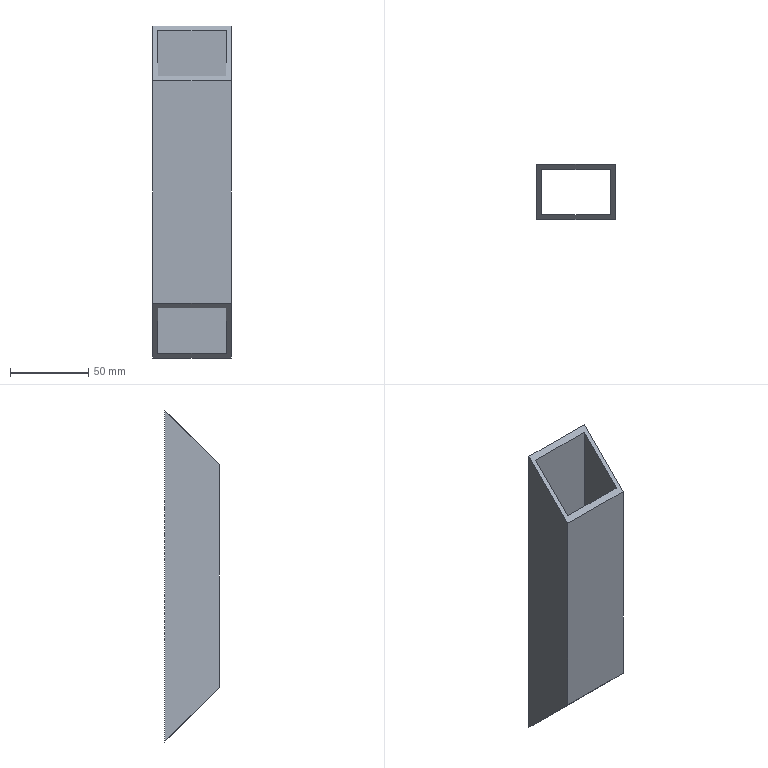Part | STEP file | BCC3 H19_7 | 1 solid | 10 faces | box 50 x 35 x 212 mm | volume 83898 mm3 | plane 10
STEP:
#1=CARTESIAN_POINT('',(0.,0.,0.));
#2=DIRECTION('',(0.,0.,1.));
#3=DIRECTION('',(1.,0.,0.));
#4=AXIS2_PLACEMENT_3D('',#1,#2,#3);
#5=CARTESIAN_POINT('',(-22.,14.5,103.));
#6=VERTEX_POINT('',#5);
#7=CARTESIAN_POINT('',(22.,14.5,103.));
#8=VERTEX_POINT('',#7);
#9=CARTESIAN_POINT('',(-22.,14.5,103.));
#10=DIRECTION('',(1.,0.,0.));
#11=VECTOR('',#10,1.);
#12=LINE('',#9,#11);
#13=CARTESIAN_POINT('',(-22.,14.5,106.));
#14=DIRECTION('',(0.,-1.,0.));
#15=DIRECTION('',(0.,0.,-1.));
#16=AXIS2_PLACEMENT_3D('',#13,#14,#15);
#17=PLANE('',#16);
#18=CARTESIAN_POINT('',(3.,0.));
#19=DIRECTION('',(0.,1.));
#20=VECTOR('',#19,1.);
#21=LINE('',#18,#20);
#22=(GEOMETRIC_REPRESENTATION_CONTEXT(2)PARAMETRIC_REPRESENTATION_CONTEXT()REPRESENTATION_CONTEXT('',''));
#23=DEFINITIONAL_REPRESENTATION('',(#21),#22);
#24=PCURVE('',#17,#23);
#25=CARTESIAN_POINT('',(-125.,-17.5,71.));
#26=DIRECTION('',(0.,0.7071,-0.7071));
#27=DIRECTION('',(0.,0.7071,0.7071));
#28=AXIS2_PLACEMENT_3D('',#25,#26,#27);
#29=PLANE('',#28);
#30=CARTESIAN_POINT('',(45.255,103.));
#31=DIRECTION('',(0.,1.));
#32=VECTOR('',#31,1.);
#33=LINE('',#30,#32);
#34=(GEOMETRIC_REPRESENTATION_CONTEXT(2)PARAMETRIC_REPRESENTATION_CONTEXT()REPRESENTATION_CONTEXT('',''));
#35=DEFINITIONAL_REPRESENTATION('',(#33),#34);
#36=PCURVE('',#29,#35);
#37=SURFACE_CURVE('',#12,(#24,#36),.PCURVE_S1.);
#38=EDGE_CURVE('',#6,#8,#37,.T.);
#39=ORIENTED_EDGE('',*,*,#38,.F.);
#40=CARTESIAN_POINT('',(-22.,14.5,-103.));
#41=VERTEX_POINT('',#40);
#42=CARTESIAN_POINT('',(-22.,14.5,106.));
#43=DIRECTION('',(0.,0.,-1.));
#44=VECTOR('',#43,1.);
#45=LINE('',#42,#44);
#46=CARTESIAN_POINT('',(0.,0.));
#47=DIRECTION('',(1.,0.));
#48=VECTOR('',#47,1.);
#49=LINE('',#46,#48);
#50=(GEOMETRIC_REPRESENTATION_CONTEXT(2)PARAMETRIC_REPRESENTATION_CONTEXT()REPRESENTATION_CONTEXT('',''));
#51=DEFINITIONAL_REPRESENTATION('',(#49),#50);
#52=PCURVE('',#17,#51);
#53=CARTESIAN_POINT('',(-22.,14.5,106.));
#54=DIRECTION('',(1.,0.,0.));
#55=DIRECTION('',(0.,1.,0.));
#56=AXIS2_PLACEMENT_3D('',#53,#54,#55);
#57=PLANE('',#56);
#58=CARTESIAN_POINT('',(0.,0.));
#59=DIRECTION('',(0.,-1.));
#60=VECTOR('',#59,1.);
#61=LINE('',#58,#60);
#62=(GEOMETRIC_REPRESENTATION_CONTEXT(2)PARAMETRIC_REPRESENTATION_CONTEXT()REPRESENTATION_CONTEXT('',''));
#63=DEFINITIONAL_REPRESENTATION('',(#61),#62);
#64=PCURVE('',#57,#63);
#65=SURFACE_CURVE('',#45,(#52,#64),.PCURVE_S1.);
#66=EDGE_CURVE('',#6,#41,#65,.T.);
#67=ORIENTED_EDGE('',*,*,#66,.T.);
#68=CARTESIAN_POINT('',(22.,14.5,-103.));
#69=VERTEX_POINT('',#68);
#70=CARTESIAN_POINT('',(-22.,14.5,-103.));
#71=DIRECTION('',(-1.,0.,0.));
#72=VECTOR('',#71,1.);
#73=LINE('',#70,#72);
#74=CARTESIAN_POINT('',(209.,0.));
#75=DIRECTION('',(0.,-1.));
#76=VECTOR('',#75,1.);
#77=LINE('',#74,#76);
#78=(GEOMETRIC_REPRESENTATION_CONTEXT(2)PARAMETRIC_REPRESENTATION_CONTEXT()REPRESENTATION_CONTEXT('',''));
#79=DEFINITIONAL_REPRESENTATION('',(#77),#78);
#80=PCURVE('',#17,#79);
#81=CARTESIAN_POINT('',(-125.,17.5,-106.));
#82=DIRECTION('',(0.,0.7071,0.7071));
#83=DIRECTION('',(0.,-0.7071,0.7071));
#84=AXIS2_PLACEMENT_3D('',#81,#82,#83);
#85=PLANE('',#84);
#86=CARTESIAN_POINT('',(4.243,103.));
#87=DIRECTION('',(0.,-1.));
#88=VECTOR('',#87,1.);
#89=LINE('',#86,#88);
#90=(GEOMETRIC_REPRESENTATION_CONTEXT(2)PARAMETRIC_REPRESENTATION_CONTEXT()REPRESENTATION_CONTEXT('',''));
#91=DEFINITIONAL_REPRESENTATION('',(#89),#90);
#92=PCURVE('',#85,#91);
#93=SURFACE_CURVE('',#73,(#80,#92),.PCURVE_S1.);
#94=EDGE_CURVE('',#69,#41,#93,.T.);
#95=ORIENTED_EDGE('',*,*,#94,.F.);
#96=CARTESIAN_POINT('',(22.,14.5,106.));
#97=DIRECTION('',(0.,0.,-1.));
#98=VECTOR('',#97,1.);
#99=LINE('',#96,#98);
#100=CARTESIAN_POINT('',(0.,44.));
#101=DIRECTION('',(1.,0.));
#102=VECTOR('',#101,1.);
#103=LINE('',#100,#102);
#104=(GEOMETRIC_REPRESENTATION_CONTEXT(2)PARAMETRIC_REPRESENTATION_CONTEXT()REPRESENTATION_CONTEXT('',''));
#105=DEFINITIONAL_REPRESENTATION('',(#103),#104);
#106=PCURVE('',#17,#105);
#107=CARTESIAN_POINT('',(22.,14.5,106.));
#108=DIRECTION('',(-1.,0.,0.));
#109=DIRECTION('',(0.,-1.,0.));
#110=AXIS2_PLACEMENT_3D('',#107,#108,#109);
#111=PLANE('',#110);
#112=CARTESIAN_POINT('',(0.,0.));
#113=DIRECTION('',(0.,-1.));
#114=VECTOR('',#113,1.);
#115=LINE('',#112,#114);
#116=(GEOMETRIC_REPRESENTATION_CONTEXT(2)PARAMETRIC_REPRESENTATION_CONTEXT()REPRESENTATION_CONTEXT('',''));
#117=DEFINITIONAL_REPRESENTATION('',(#115),#116);
#118=PCURVE('',#111,#117);
#119=SURFACE_CURVE('',#99,(#106,#118),.PCURVE_S1.);
#120=EDGE_CURVE('',#8,#69,#119,.T.);
#121=ORIENTED_EDGE('',*,*,#120,.F.);
#122=EDGE_LOOP('',(#39,#67,#95,#121));
#123=FACE_BOUND('',#122,.T.);
#124=ADVANCED_FACE('',(#123),#17,.T.);
#125=CARTESIAN_POINT('',(22.,-14.5,74.));
#126=VERTEX_POINT('',#125);
#127=CARTESIAN_POINT('',(22.,16.,104.5));
#128=DIRECTION('',(0.,-0.7071,-0.7071));
#129=VECTOR('',#128,1.);
#130=LINE('',#127,#129);
#131=CARTESIAN_POINT('',(-1.5,-1.5));
#132=DIRECTION('',(0.7071,-0.7071));
#133=VECTOR('',#132,1.);
#134=LINE('',#131,#133);
#135=(GEOMETRIC_REPRESENTATION_CONTEXT(2)PARAMETRIC_REPRESENTATION_CONTEXT()REPRESENTATION_CONTEXT('',''));
#136=DEFINITIONAL_REPRESENTATION('',(#134),#135);
#137=PCURVE('',#111,#136);
#138=CARTESIAN_POINT('',(47.376,147.));
#139=DIRECTION('',(-1.,0.));
#140=VECTOR('',#139,1.);
#141=LINE('',#138,#140);
#142=(GEOMETRIC_REPRESENTATION_CONTEXT(2)PARAMETRIC_REPRESENTATION_CONTEXT()REPRESENTATION_CONTEXT('',''));
#143=DEFINITIONAL_REPRESENTATION('',(#141),#142);
#144=PCURVE('',#29,#143);
#145=SURFACE_CURVE('',#130,(#137,#144),.PCURVE_S1.);
#146=EDGE_CURVE('',#8,#126,#145,.T.);
#147=ORIENTED_EDGE('',*,*,#146,.F.);
#148=ORIENTED_EDGE('',*,*,#120,.T.);
#149=CARTESIAN_POINT('',(22.,-14.5,-74.));
#150=VERTEX_POINT('',#149);
#151=CARTESIAN_POINT('',(22.,-90.,1.5));
#152=DIRECTION('',(0.,0.7071,-0.7071));
#153=VECTOR('',#152,1.);
#154=LINE('',#151,#153);
#155=CARTESIAN_POINT('',(104.5,-104.5));
#156=DIRECTION('',(-0.7071,-0.7071));
#157=VECTOR('',#156,1.);
#158=LINE('',#155,#157);
#159=(GEOMETRIC_REPRESENTATION_CONTEXT(2)PARAMETRIC_REPRESENTATION_CONTEXT()REPRESENTATION_CONTEXT('',''));
#160=DEFINITIONAL_REPRESENTATION('',(#158),#159);
#161=PCURVE('',#111,#160);
#162=CARTESIAN_POINT('',(152.028,147.));
#163=DIRECTION('',(-1.,0.));
#164=VECTOR('',#163,1.);
#165=LINE('',#162,#164);
#166=(GEOMETRIC_REPRESENTATION_CONTEXT(2)PARAMETRIC_REPRESENTATION_CONTEXT()REPRESENTATION_CONTEXT('',''));
#167=DEFINITIONAL_REPRESENTATION('',(#165),#166);
#168=PCURVE('',#85,#167);
#169=SURFACE_CURVE('',#154,(#161,#168),.PCURVE_S1.);
#170=EDGE_CURVE('',#150,#69,#169,.T.);
#171=ORIENTED_EDGE('',*,*,#170,.F.);
#172=CARTESIAN_POINT('',(22.,-14.5,106.));
#173=DIRECTION('',(0.,0.,-1.));
#174=VECTOR('',#173,1.);
#175=LINE('',#172,#174);
#176=CARTESIAN_POINT('',(29.,0.));
#177=DIRECTION('',(0.,-1.));
#178=VECTOR('',#177,1.);
#179=LINE('',#176,#178);
#180=(GEOMETRIC_REPRESENTATION_CONTEXT(2)PARAMETRIC_REPRESENTATION_CONTEXT()REPRESENTATION_CONTEXT('',''));
#181=DEFINITIONAL_REPRESENTATION('',(#179),#180);
#182=PCURVE('',#111,#181);
#183=CARTESIAN_POINT('',(-22.,-14.5,106.));
#184=DIRECTION('',(0.,1.,0.));
#185=DIRECTION('',(0.,0.,1.));
#186=AXIS2_PLACEMENT_3D('',#183,#184,#185);
#187=PLANE('',#186);
#188=CARTESIAN_POINT('',(0.,44.));
#189=DIRECTION('',(-1.,0.));
#190=VECTOR('',#189,1.);
#191=LINE('',#188,#190);
#192=(GEOMETRIC_REPRESENTATION_CONTEXT(2)PARAMETRIC_REPRESENTATION_CONTEXT()REPRESENTATION_CONTEXT('',''));
#193=DEFINITIONAL_REPRESENTATION('',(#191),#192);
#194=PCURVE('',#187,#193);
#195=SURFACE_CURVE('',#175,(#182,#194),.PCURVE_S1.);
#196=EDGE_CURVE('',#126,#150,#195,.T.);
#197=ORIENTED_EDGE('',*,*,#196,.F.);
#198=EDGE_LOOP('',(#147,#148,#171,#197));
#199=FACE_BOUND('',#198,.T.);
#200=ADVANCED_FACE('',(#199),#111,.T.);
#201=CARTESIAN_POINT('',(-22.,-14.5,74.));
#202=VERTEX_POINT('',#201);
#203=CARTESIAN_POINT('',(-22.,-14.5,74.));
#204=DIRECTION('',(-1.,0.,0.));
#205=VECTOR('',#204,1.);
#206=LINE('',#203,#205);
#207=CARTESIAN_POINT('',(-32.,0.));
#208=DIRECTION('',(0.,-1.));
#209=VECTOR('',#208,1.);
#210=LINE('',#207,#209);
#211=(GEOMETRIC_REPRESENTATION_CONTEXT(2)PARAMETRIC_REPRESENTATION_CONTEXT()REPRESENTATION_CONTEXT('',''));
#212=DEFINITIONAL_REPRESENTATION('',(#210),#211);
#213=PCURVE('',#187,#212);
#214=CARTESIAN_POINT('',(4.243,103.));
#215=DIRECTION('',(0.,-1.));
#216=VECTOR('',#215,1.);
#217=LINE('',#214,#216);
#218=(GEOMETRIC_REPRESENTATION_CONTEXT(2)PARAMETRIC_REPRESENTATION_CONTEXT()REPRESENTATION_CONTEXT('',''));
#219=DEFINITIONAL_REPRESENTATION('',(#217),#218);
#220=PCURVE('',#29,#219);
#221=SURFACE_CURVE('',#206,(#213,#220),.PCURVE_S1.);
#222=EDGE_CURVE('',#126,#202,#221,.T.);
#223=ORIENTED_EDGE('',*,*,#222,.F.);
#224=ORIENTED_EDGE('',*,*,#196,.T.);
#225=CARTESIAN_POINT('',(-22.,-14.5,-74.));
#226=VERTEX_POINT('',#225);
#227=CARTESIAN_POINT('',(-22.,-14.5,-74.));
#228=DIRECTION('',(1.,0.,0.));
#229=VECTOR('',#228,1.);
#230=LINE('',#227,#229);
#231=CARTESIAN_POINT('',(-180.,0.));
#232=DIRECTION('',(0.,1.));
#233=VECTOR('',#232,1.);
#234=LINE('',#231,#233);
#235=(GEOMETRIC_REPRESENTATION_CONTEXT(2)PARAMETRIC_REPRESENTATION_CONTEXT()REPRESENTATION_CONTEXT('',''));
#236=DEFINITIONAL_REPRESENTATION('',(#234),#235);
#237=PCURVE('',#187,#236);
#238=CARTESIAN_POINT('',(45.255,103.));
#239=DIRECTION('',(0.,1.));
#240=VECTOR('',#239,1.);
#241=LINE('',#238,#240);
#242=(GEOMETRIC_REPRESENTATION_CONTEXT(2)PARAMETRIC_REPRESENTATION_CONTEXT()REPRESENTATION_CONTEXT('',''));
#243=DEFINITIONAL_REPRESENTATION('',(#241),#242);
#244=PCURVE('',#85,#243);
#245=SURFACE_CURVE('',#230,(#237,#244),.PCURVE_S1.);
#246=EDGE_CURVE('',#226,#150,#245,.T.);
#247=ORIENTED_EDGE('',*,*,#246,.F.);
#248=CARTESIAN_POINT('',(-22.,-14.5,106.));
#249=DIRECTION('',(0.,0.,-1.));
#250=VECTOR('',#249,1.);
#251=LINE('',#248,#250);
#252=CARTESIAN_POINT('',(0.,0.));
#253=DIRECTION('',(-1.,0.));
#254=VECTOR('',#253,1.);
#255=LINE('',#252,#254);
#256=(GEOMETRIC_REPRESENTATION_CONTEXT(2)PARAMETRIC_REPRESENTATION_CONTEXT()REPRESENTATION_CONTEXT('',''));
#257=DEFINITIONAL_REPRESENTATION('',(#255),#256);
#258=PCURVE('',#187,#257);
#259=CARTESIAN_POINT('',(-29.,0.));
#260=DIRECTION('',(0.,-1.));
#261=VECTOR('',#260,1.);
#262=LINE('',#259,#261);
#263=(GEOMETRIC_REPRESENTATION_CONTEXT(2)PARAMETRIC_REPRESENTATION_CONTEXT()REPRESENTATION_CONTEXT('',''));
#264=DEFINITIONAL_REPRESENTATION('',(#262),#263);
#265=PCURVE('',#57,#264);
#266=SURFACE_CURVE('',#251,(#258,#265),.PCURVE_S1.);
#267=EDGE_CURVE('',#202,#226,#266,.T.);
#268=ORIENTED_EDGE('',*,*,#267,.F.);
#269=EDGE_LOOP('',(#223,#224,#247,#268));
#270=FACE_BOUND('',#269,.T.);
#271=ADVANCED_FACE('',(#270),#187,.T.);
#272=CARTESIAN_POINT('',(-22.,16.,104.5));
#273=DIRECTION('',(0.,0.7071,0.7071));
#274=VECTOR('',#273,1.);
#275=LINE('',#272,#274);
#276=CARTESIAN_POINT('',(1.5,-1.5));
#277=DIRECTION('',(0.7071,0.7071));
#278=VECTOR('',#277,1.);
#279=LINE('',#276,#278);
#280=(GEOMETRIC_REPRESENTATION_CONTEXT(2)PARAMETRIC_REPRESENTATION_CONTEXT()REPRESENTATION_CONTEXT('',''));
#281=DEFINITIONAL_REPRESENTATION('',(#279),#280);
#282=PCURVE('',#57,#281);
#283=CARTESIAN_POINT('',(47.376,103.));
#284=DIRECTION('',(1.,0.));
#285=VECTOR('',#284,1.);
#286=LINE('',#283,#285);
#287=(GEOMETRIC_REPRESENTATION_CONTEXT(2)PARAMETRIC_REPRESENTATION_CONTEXT()REPRESENTATION_CONTEXT('',''));
#288=DEFINITIONAL_REPRESENTATION('',(#286),#287);
#289=PCURVE('',#29,#288);
#290=SURFACE_CURVE('',#275,(#282,#289),.PCURVE_S1.);
#291=EDGE_CURVE('',#202,#6,#290,.T.);
#292=ORIENTED_EDGE('',*,*,#291,.F.);
#293=ORIENTED_EDGE('',*,*,#267,.T.);
#294=CARTESIAN_POINT('',(-22.,-90.,1.5));
#295=DIRECTION('',(0.,-0.7071,0.7071));
#296=VECTOR('',#295,1.);
#297=LINE('',#294,#296);
#298=CARTESIAN_POINT('',(-104.5,-104.5));
#299=DIRECTION('',(-0.7071,0.7071));
#300=VECTOR('',#299,1.);
#301=LINE('',#298,#300);
#302=(GEOMETRIC_REPRESENTATION_CONTEXT(2)PARAMETRIC_REPRESENTATION_CONTEXT()REPRESENTATION_CONTEXT('',''));
#303=DEFINITIONAL_REPRESENTATION('',(#301),#302);
#304=PCURVE('',#57,#303);
#305=CARTESIAN_POINT('',(152.028,103.));
#306=DIRECTION('',(1.,0.));
#307=VECTOR('',#306,1.);
#308=LINE('',#305,#307);
#309=(GEOMETRIC_REPRESENTATION_CONTEXT(2)PARAMETRIC_REPRESENTATION_CONTEXT()REPRESENTATION_CONTEXT('',''));
#310=DEFINITIONAL_REPRESENTATION('',(#308),#309);
#311=PCURVE('',#85,#310);
#312=SURFACE_CURVE('',#297,(#304,#311),.PCURVE_S1.);
#313=EDGE_CURVE('',#41,#226,#312,.T.);
#314=ORIENTED_EDGE('',*,*,#313,.F.);
#315=ORIENTED_EDGE('',*,*,#66,.F.);
#316=EDGE_LOOP('',(#292,#293,#314,#315));
#317=FACE_BOUND('',#316,.T.);
#318=ADVANCED_FACE('',(#317),#57,.T.);
#319=ORIENTED_EDGE('',*,*,#313,.T.);
#320=ORIENTED_EDGE('',*,*,#246,.T.);
#321=ORIENTED_EDGE('',*,*,#170,.T.);
#322=ORIENTED_EDGE('',*,*,#94,.T.);
#323=EDGE_LOOP('',(#319,#320,#321,#322));
#324=FACE_BOUND('',#323,.T.);
#325=CARTESIAN_POINT('',(25.,17.5,-106.));
#326=VERTEX_POINT('',#325);
#327=CARTESIAN_POINT('',(-25.,17.5,-106.));
#328=VERTEX_POINT('',#327);
#329=CARTESIAN_POINT('',(-25.,17.5,-106.));
#330=DIRECTION('',(-1.,0.,0.));
#331=VECTOR('',#330,1.);
#332=LINE('',#329,#331);
#333=CARTESIAN_POINT('',(0.,100.));
#334=DIRECTION('',(0.,-1.));
#335=VECTOR('',#334,1.);
#336=LINE('',#333,#335);
#337=(GEOMETRIC_REPRESENTATION_CONTEXT(2)PARAMETRIC_REPRESENTATION_CONTEXT()REPRESENTATION_CONTEXT('',''));
#338=DEFINITIONAL_REPRESENTATION('',(#336),#337);
#339=PCURVE('',#85,#338);
#340=CARTESIAN_POINT('',(-25.,17.5,106.));
#341=DIRECTION('',(0.,-1.,0.));
#342=DIRECTION('',(0.,0.,-1.));
#343=AXIS2_PLACEMENT_3D('',#340,#341,#342);
#344=PLANE('',#343);
#345=CARTESIAN_POINT('',(212.,0.));
#346=DIRECTION('',(0.,-1.));
#347=VECTOR('',#346,1.);
#348=LINE('',#345,#347);
#349=(GEOMETRIC_REPRESENTATION_CONTEXT(2)PARAMETRIC_REPRESENTATION_CONTEXT()REPRESENTATION_CONTEXT('',''));
#350=DEFINITIONAL_REPRESENTATION('',(#348),#349);
#351=PCURVE('',#344,#350);
#352=SURFACE_CURVE('',#332,(#339,#351),.PCURVE_S1.);
#353=EDGE_CURVE('',#326,#328,#352,.T.);
#354=ORIENTED_EDGE('',*,*,#353,.F.);
#355=CARTESIAN_POINT('',(25.,-17.5,-71.));
#356=VERTEX_POINT('',#355);
#357=CARTESIAN_POINT('',(25.,17.5,-106.));
#358=DIRECTION('',(0.,-0.7071,0.7071));
#359=VECTOR('',#358,1.);
#360=LINE('',#357,#359);
#361=CARTESIAN_POINT('',(0.,150.));
#362=DIRECTION('',(1.,0.));
#363=VECTOR('',#362,1.);
#364=LINE('',#361,#363);
#365=(GEOMETRIC_REPRESENTATION_CONTEXT(2)PARAMETRIC_REPRESENTATION_CONTEXT()REPRESENTATION_CONTEXT('',''));
#366=DEFINITIONAL_REPRESENTATION('',(#364),#365);
#367=PCURVE('',#85,#366);
#368=CARTESIAN_POINT('',(25.,17.5,106.));
#369=DIRECTION('',(-1.,0.,0.));
#370=DIRECTION('',(0.,-1.,0.));
#371=AXIS2_PLACEMENT_3D('',#368,#369,#370);
#372=PLANE('',#371);
#373=CARTESIAN_POINT('',(0.,-212.));
#374=DIRECTION('',(0.7071,0.7071));
#375=VECTOR('',#374,1.);
#376=LINE('',#373,#375);
#377=(GEOMETRIC_REPRESENTATION_CONTEXT(2)PARAMETRIC_REPRESENTATION_CONTEXT()REPRESENTATION_CONTEXT('',''));
#378=DEFINITIONAL_REPRESENTATION('',(#376),#377);
#379=PCURVE('',#372,#378);
#380=SURFACE_CURVE('',#360,(#367,#379),.PCURVE_S1.);
#381=EDGE_CURVE('',#326,#356,#380,.T.);
#382=ORIENTED_EDGE('',*,*,#381,.T.);
#383=CARTESIAN_POINT('',(-25.,-17.5,-71.));
#384=VERTEX_POINT('',#383);
#385=CARTESIAN_POINT('',(-125.,-17.5,-71.));
#386=DIRECTION('',(1.,0.,0.));
#387=VECTOR('',#386,1.);
#388=LINE('',#385,#387);
#389=CARTESIAN_POINT('',(49.497,0.));
#390=DIRECTION('',(0.,1.));
#391=VECTOR('',#390,1.);
#392=LINE('',#389,#391);
#393=(GEOMETRIC_REPRESENTATION_CONTEXT(2)PARAMETRIC_REPRESENTATION_CONTEXT()REPRESENTATION_CONTEXT('',''));
#394=DEFINITIONAL_REPRESENTATION('',(#392),#393);
#395=PCURVE('',#85,#394);
#396=CARTESIAN_POINT('',(-25.,-17.5,106.));
#397=DIRECTION('',(0.,1.,0.));
#398=DIRECTION('',(0.,0.,1.));
#399=AXIS2_PLACEMENT_3D('',#396,#397,#398);
#400=PLANE('',#399);
#401=CARTESIAN_POINT('',(-177.,-100.));
#402=DIRECTION('',(0.,1.));
#403=VECTOR('',#402,1.);
#404=LINE('',#401,#403);
#405=(GEOMETRIC_REPRESENTATION_CONTEXT(2)PARAMETRIC_REPRESENTATION_CONTEXT()REPRESENTATION_CONTEXT('',''));
#406=DEFINITIONAL_REPRESENTATION('',(#404),#405);
#407=PCURVE('',#400,#406);
#408=SURFACE_CURVE('',#388,(#395,#407),.PCURVE_S1.);
#409=EDGE_CURVE('',#384,#356,#408,.T.);
#410=ORIENTED_EDGE('',*,*,#409,.F.);
#411=CARTESIAN_POINT('',(-25.,-88.5,0.));
#412=DIRECTION('',(0.,-0.7071,0.7071));
#413=VECTOR('',#412,1.);
#414=LINE('',#411,#413);
#415=CARTESIAN_POINT('',(149.907,100.));
#416=DIRECTION('',(1.,0.));
#417=VECTOR('',#416,1.);
#418=LINE('',#415,#417);
#419=(GEOMETRIC_REPRESENTATION_CONTEXT(2)PARAMETRIC_REPRESENTATION_CONTEXT()REPRESENTATION_CONTEXT('',''));
#420=DEFINITIONAL_REPRESENTATION('',(#418),#419);
#421=PCURVE('',#85,#420);
#422=CARTESIAN_POINT('',(-25.,17.5,106.));
#423=DIRECTION('',(1.,0.,0.));
#424=DIRECTION('',(0.,1.,0.));
#425=AXIS2_PLACEMENT_3D('',#422,#423,#424);
#426=PLANE('',#425);
#427=CARTESIAN_POINT('',(-106.,-106.));
#428=DIRECTION('',(-0.7071,0.7071));
#429=VECTOR('',#428,1.);
#430=LINE('',#427,#429);
#431=(GEOMETRIC_REPRESENTATION_CONTEXT(2)PARAMETRIC_REPRESENTATION_CONTEXT()REPRESENTATION_CONTEXT('',''));
#432=DEFINITIONAL_REPRESENTATION('',(#430),#431);
#433=PCURVE('',#426,#432);
#434=SURFACE_CURVE('',#414,(#421,#433),.PCURVE_S1.);
#435=EDGE_CURVE('',#328,#384,#434,.T.);
#436=ORIENTED_EDGE('',*,*,#435,.F.);
#437=EDGE_LOOP('',(#354,#382,#410,#436));
#438=FACE_BOUND('',#437,.T.);
#439=ADVANCED_FACE('',(#324,#438),#85,.F.);
#440=ORIENTED_EDGE('',*,*,#291,.T.);
#441=ORIENTED_EDGE('',*,*,#38,.T.);
#442=ORIENTED_EDGE('',*,*,#146,.T.);
#443=ORIENTED_EDGE('',*,*,#222,.T.);
#444=EDGE_LOOP('',(#440,#441,#442,#443));
#445=FACE_BOUND('',#444,.T.);
#446=CARTESIAN_POINT('',(-25.,-17.5,71.));
#447=VERTEX_POINT('',#446);
#448=CARTESIAN_POINT('',(25.,-17.5,71.));
#449=VERTEX_POINT('',#448);
#450=CARTESIAN_POINT('',(-125.,-17.5,71.));
#451=DIRECTION('',(1.,0.,0.));
#452=VECTOR('',#451,1.);
#453=LINE('',#450,#452);
#454=CARTESIAN_POINT('',(0.,0.));
#455=DIRECTION('',(0.,1.));
#456=VECTOR('',#455,1.);
#457=LINE('',#454,#456);
#458=(GEOMETRIC_REPRESENTATION_CONTEXT(2)PARAMETRIC_REPRESENTATION_CONTEXT()REPRESENTATION_CONTEXT('',''));
#459=DEFINITIONAL_REPRESENTATION('',(#457),#458);
#460=PCURVE('',#29,#459);
#461=CARTESIAN_POINT('',(-35.,-100.));
#462=DIRECTION('',(0.,1.));
#463=VECTOR('',#462,1.);
#464=LINE('',#461,#463);
#465=(GEOMETRIC_REPRESENTATION_CONTEXT(2)PARAMETRIC_REPRESENTATION_CONTEXT()REPRESENTATION_CONTEXT('',''));
#466=DEFINITIONAL_REPRESENTATION('',(#464),#465);
#467=PCURVE('',#400,#466);
#468=SURFACE_CURVE('',#453,(#460,#467),.PCURVE_S1.);
#469=EDGE_CURVE('',#447,#449,#468,.T.);
#470=ORIENTED_EDGE('',*,*,#469,.T.);
#471=CARTESIAN_POINT('',(25.,17.5,106.));
#472=VERTEX_POINT('',#471);
#473=CARTESIAN_POINT('',(25.,-17.5,71.));
#474=DIRECTION('',(0.,0.7071,0.7071));
#475=VECTOR('',#474,1.);
#476=LINE('',#473,#475);
#477=CARTESIAN_POINT('',(0.,150.));
#478=DIRECTION('',(1.,0.));
#479=VECTOR('',#478,1.);
#480=LINE('',#477,#479);
#481=(GEOMETRIC_REPRESENTATION_CONTEXT(2)PARAMETRIC_REPRESENTATION_CONTEXT()REPRESENTATION_CONTEXT('',''));
#482=DEFINITIONAL_REPRESENTATION('',(#480),#481);
#483=PCURVE('',#29,#482);
#484=CARTESIAN_POINT('',(35.,-35.));
#485=DIRECTION('',(-0.7071,0.7071));
#486=VECTOR('',#485,1.);
#487=LINE('',#484,#486);
#488=(GEOMETRIC_REPRESENTATION_CONTEXT(2)PARAMETRIC_REPRESENTATION_CONTEXT()REPRESENTATION_CONTEXT('',''));
#489=DEFINITIONAL_REPRESENTATION('',(#487),#488);
#490=PCURVE('',#372,#489);
#491=SURFACE_CURVE('',#476,(#483,#490),.PCURVE_S1.);
#492=EDGE_CURVE('',#449,#472,#491,.T.);
#493=ORIENTED_EDGE('',*,*,#492,.T.);
#494=CARTESIAN_POINT('',(-25.,17.5,106.));
#495=VERTEX_POINT('',#494);
#496=CARTESIAN_POINT('',(-25.,17.5,106.));
#497=DIRECTION('',(-1.,0.,0.));
#498=VECTOR('',#497,1.);
#499=LINE('',#496,#498);
#500=CARTESIAN_POINT('',(49.497,100.));
#501=DIRECTION('',(0.,-1.));
#502=VECTOR('',#501,1.);
#503=LINE('',#500,#502);
#504=(GEOMETRIC_REPRESENTATION_CONTEXT(2)PARAMETRIC_REPRESENTATION_CONTEXT()REPRESENTATION_CONTEXT('',''));
#505=DEFINITIONAL_REPRESENTATION('',(#503),#504);
#506=PCURVE('',#29,#505);
#507=CARTESIAN_POINT('',(0.,0.));
#508=DIRECTION('',(0.,-1.));
#509=VECTOR('',#508,1.);
#510=LINE('',#507,#509);
#511=(GEOMETRIC_REPRESENTATION_CONTEXT(2)PARAMETRIC_REPRESENTATION_CONTEXT()REPRESENTATION_CONTEXT('',''));
#512=DEFINITIONAL_REPRESENTATION('',(#510),#511);
#513=PCURVE('',#344,#512);
#514=SURFACE_CURVE('',#499,(#506,#513),.PCURVE_S1.);
#515=EDGE_CURVE('',#472,#495,#514,.T.);
#516=ORIENTED_EDGE('',*,*,#515,.T.);
#517=CARTESIAN_POINT('',(-25.,17.5,106.));
#518=DIRECTION('',(0.,0.7071,0.7071));
#519=VECTOR('',#518,1.);
#520=LINE('',#517,#519);
#521=CARTESIAN_POINT('',(49.497,100.));
#522=DIRECTION('',(1.,0.));
#523=VECTOR('',#522,1.);
#524=LINE('',#521,#523);
#525=(GEOMETRIC_REPRESENTATION_CONTEXT(2)PARAMETRIC_REPRESENTATION_CONTEXT()REPRESENTATION_CONTEXT('',''));
#526=DEFINITIONAL_REPRESENTATION('',(#524),#525);
#527=PCURVE('',#29,#526);
#528=CARTESIAN_POINT('',(0.,0.));
#529=DIRECTION('',(0.7071,0.7071));
#530=VECTOR('',#529,1.);
#531=LINE('',#528,#530);
#532=(GEOMETRIC_REPRESENTATION_CONTEXT(2)PARAMETRIC_REPRESENTATION_CONTEXT()REPRESENTATION_CONTEXT('',''));
#533=DEFINITIONAL_REPRESENTATION('',(#531),#532);
#534=PCURVE('',#426,#533);
#535=SURFACE_CURVE('',#520,(#527,#534),.PCURVE_S1.);
#536=EDGE_CURVE('',#447,#495,#535,.T.);
#537=ORIENTED_EDGE('',*,*,#536,.F.);
#538=EDGE_LOOP('',(#470,#493,#516,#537));
#539=FACE_BOUND('',#538,.T.);
#540=ADVANCED_FACE('',(#445,#539),#29,.F.);
#541=CARTESIAN_POINT('',(-25.,-17.5,106.));
#542=DIRECTION('',(0.,0.,-1.));
#543=VECTOR('',#542,1.);
#544=LINE('',#541,#543);
#545=CARTESIAN_POINT('',(-35.,0.));
#546=DIRECTION('',(0.,-1.));
#547=VECTOR('',#546,1.);
#548=LINE('',#545,#547);
#549=(GEOMETRIC_REPRESENTATION_CONTEXT(2)PARAMETRIC_REPRESENTATION_CONTEXT()REPRESENTATION_CONTEXT('',''));
#550=DEFINITIONAL_REPRESENTATION('',(#548),#549);
#551=PCURVE('',#426,#550);
#552=CARTESIAN_POINT('',(0.,0.));
#553=DIRECTION('',(-1.,0.));
#554=VECTOR('',#553,1.);
#555=LINE('',#552,#554);
#556=(GEOMETRIC_REPRESENTATION_CONTEXT(2)PARAMETRIC_REPRESENTATION_CONTEXT()REPRESENTATION_CONTEXT('',''));
#557=DEFINITIONAL_REPRESENTATION('',(#555),#556);
#558=PCURVE('',#400,#557);
#559=SURFACE_CURVE('',#544,(#551,#558),.PCURVE_S1.);
#560=EDGE_CURVE('',#447,#384,#559,.T.);
#561=ORIENTED_EDGE('',*,*,#560,.F.);
#562=ORIENTED_EDGE('',*,*,#536,.T.);
#563=CARTESIAN_POINT('',(-25.,17.5,106.));
#564=DIRECTION('',(0.,0.,-1.));
#565=VECTOR('',#564,1.);
#566=LINE('',#563,#565);
#567=CARTESIAN_POINT('',(0.,0.));
#568=DIRECTION('',(0.,-1.));
#569=VECTOR('',#568,1.);
#570=LINE('',#567,#569);
#571=(GEOMETRIC_REPRESENTATION_CONTEXT(2)PARAMETRIC_REPRESENTATION_CONTEXT()REPRESENTATION_CONTEXT('',''));
#572=DEFINITIONAL_REPRESENTATION('',(#570),#571);
#573=PCURVE('',#426,#572);
#574=CARTESIAN_POINT('',(0.,0.));
#575=DIRECTION('',(1.,0.));
#576=VECTOR('',#575,1.);
#577=LINE('',#574,#576);
#578=(GEOMETRIC_REPRESENTATION_CONTEXT(2)PARAMETRIC_REPRESENTATION_CONTEXT()REPRESENTATION_CONTEXT('',''));
#579=DEFINITIONAL_REPRESENTATION('',(#577),#578);
#580=PCURVE('',#344,#579);
#581=SURFACE_CURVE('',#566,(#573,#580),.PCURVE_S1.);
#582=EDGE_CURVE('',#495,#328,#581,.T.);
#583=ORIENTED_EDGE('',*,*,#582,.T.);
#584=ORIENTED_EDGE('',*,*,#435,.T.);
#585=EDGE_LOOP('',(#561,#562,#583,#584));
#586=FACE_BOUND('',#585,.T.);
#587=ADVANCED_FACE('',(#586),#426,.F.);
#588=CARTESIAN_POINT('',(25.,-17.5,106.));
#589=DIRECTION('',(0.,0.,-1.));
#590=VECTOR('',#589,1.);
#591=LINE('',#588,#590);
#592=CARTESIAN_POINT('',(0.,50.));
#593=DIRECTION('',(-1.,0.));
#594=VECTOR('',#593,1.);
#595=LINE('',#592,#594);
#596=(GEOMETRIC_REPRESENTATION_CONTEXT(2)PARAMETRIC_REPRESENTATION_CONTEXT()REPRESENTATION_CONTEXT('',''));
#597=DEFINITIONAL_REPRESENTATION('',(#595),#596);
#598=PCURVE('',#400,#597);
#599=CARTESIAN_POINT('',(35.,0.));
#600=DIRECTION('',(0.,-1.));
#601=VECTOR('',#600,1.);
#602=LINE('',#599,#601);
#603=(GEOMETRIC_REPRESENTATION_CONTEXT(2)PARAMETRIC_REPRESENTATION_CONTEXT()REPRESENTATION_CONTEXT('',''));
#604=DEFINITIONAL_REPRESENTATION('',(#602),#603);
#605=PCURVE('',#372,#604);
#606=SURFACE_CURVE('',#591,(#598,#605),.PCURVE_S1.);
#607=EDGE_CURVE('',#449,#356,#606,.T.);
#608=ORIENTED_EDGE('',*,*,#607,.F.);
#609=ORIENTED_EDGE('',*,*,#469,.F.);
#610=ORIENTED_EDGE('',*,*,#560,.T.);
#611=ORIENTED_EDGE('',*,*,#409,.T.);
#612=EDGE_LOOP('',(#608,#609,#610,#611));
#613=FACE_BOUND('',#612,.T.);
#614=ADVANCED_FACE('',(#613),#400,.F.);
#615=CARTESIAN_POINT('',(25.,17.5,106.));
#616=DIRECTION('',(0.,0.,-1.));
#617=VECTOR('',#616,1.);
#618=LINE('',#615,#617);
#619=CARTESIAN_POINT('',(0.,0.));
#620=DIRECTION('',(0.,-1.));
#621=VECTOR('',#620,1.);
#622=LINE('',#619,#621);
#623=(GEOMETRIC_REPRESENTATION_CONTEXT(2)PARAMETRIC_REPRESENTATION_CONTEXT()REPRESENTATION_CONTEXT('',''));
#624=DEFINITIONAL_REPRESENTATION('',(#622),#623);
#625=PCURVE('',#372,#624);
#626=CARTESIAN_POINT('',(0.,50.));
#627=DIRECTION('',(1.,0.));
#628=VECTOR('',#627,1.);
#629=LINE('',#626,#628);
#630=(GEOMETRIC_REPRESENTATION_CONTEXT(2)PARAMETRIC_REPRESENTATION_CONTEXT()REPRESENTATION_CONTEXT('',''));
#631=DEFINITIONAL_REPRESENTATION('',(#629),#630);
#632=PCURVE('',#344,#631);
#633=SURFACE_CURVE('',#618,(#625,#632),.PCURVE_S1.);
#634=EDGE_CURVE('',#472,#326,#633,.T.);
#635=ORIENTED_EDGE('',*,*,#634,.F.);
#636=ORIENTED_EDGE('',*,*,#492,.F.);
#637=ORIENTED_EDGE('',*,*,#607,.T.);
#638=ORIENTED_EDGE('',*,*,#381,.F.);
#639=EDGE_LOOP('',(#635,#636,#637,#638));
#640=FACE_BOUND('',#639,.T.);
#641=ADVANCED_FACE('',(#640),#372,.F.);
#642=ORIENTED_EDGE('',*,*,#353,.T.);
#643=ORIENTED_EDGE('',*,*,#582,.F.);
#644=ORIENTED_EDGE('',*,*,#515,.F.);
#645=ORIENTED_EDGE('',*,*,#634,.T.);
#646=EDGE_LOOP('',(#642,#643,#644,#645));
#647=FACE_BOUND('',#646,.T.);
#648=ADVANCED_FACE('',(#647),#344,.F.);
#649=CLOSED_SHELL('',(#124,#200,#271,#318,#439,#540,#587,#614,#641,#648));
#650=MANIFOLD_SOLID_BREP('',#649);
#651=(LENGTH_UNIT()NAMED_UNIT(*)SI_UNIT(.MILLI.,.METRE.));
#652=UNCERTAINTY_MEASURE_WITH_UNIT(LENGTH_MEASURE(0.0000001),#651,'','');
#653=(NAMED_UNIT(*)PLANE_ANGLE_UNIT()SI_UNIT($,.RADIAN.));
#654=(NAMED_UNIT(*)SI_UNIT($,.STERADIAN.)SOLID_ANGLE_UNIT());
#655=(GEOMETRIC_REPRESENTATION_CONTEXT(3)GLOBAL_UNCERTAINTY_ASSIGNED_CONTEXT((#652))GLOBAL_UNIT_ASSIGNED_CONTEXT((#651,#653,#654))REPRESENTATION_CONTEXT('',''));
#656=ADVANCED_BREP_SHAPE_REPRESENTATION('',(#4,#650),#655);